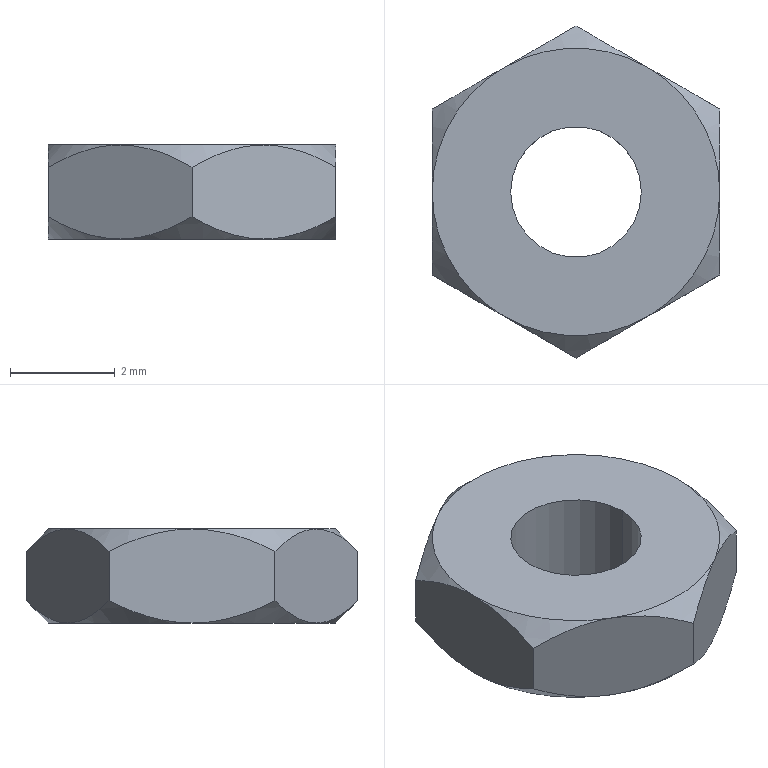Part | NX | 1 solid | 22 faces | box 5.5 x 6.351 x 1.8 mm | volume 37.693 mm3 | cone 12 | plane 8 | cylinder 2 | commonest cylinder face diameters 2.5 x2
STEP:
#1=CARTESIAN_POINT('',(1.375,-2.382,-0.9));
#2=VERTEX_POINT('',#1);
#3=CARTESIAN_POINT('',(2.75,0.,-0.9));
#4=VERTEX_POINT('',#3);
#5=CARTESIAN_POINT('',(0.,0.,-0.9));
#6=DIRECTION('',(0.,0.,1.));
#7=DIRECTION('',(0.5,-0.866,0.));
#8=AXIS2_PLACEMENT_3D('',#5,#6,#7);
#9=CIRCLE('',#8,2.75);
#10=EDGE_CURVE('',#2,#4,#9,.T.);
#11=ORIENTED_EDGE('',*,*,#10,.F.);
#12=CARTESIAN_POINT('',(-1.375,-2.382,-0.9));
#13=VERTEX_POINT('',#12);
#14=CARTESIAN_POINT('',(0.,0.,-0.9));
#15=DIRECTION('',(0.,0.,1.));
#16=DIRECTION('',(-0.5,-0.866,0.));
#17=AXIS2_PLACEMENT_3D('',#14,#15,#16);
#18=CIRCLE('',#17,2.75);
#19=EDGE_CURVE('',#13,#2,#18,.T.);
#20=ORIENTED_EDGE('',*,*,#19,.F.);
#21=CARTESIAN_POINT('',(-2.75,0.,-0.9));
#22=VERTEX_POINT('',#21);
#23=CARTESIAN_POINT('',(0.,0.,-0.9));
#24=DIRECTION('',(0.,0.,1.));
#25=DIRECTION('',(-1.,0.,0.));
#26=AXIS2_PLACEMENT_3D('',#23,#24,#25);
#27=CIRCLE('',#26,2.75);
#28=EDGE_CURVE('',#22,#13,#27,.T.);
#29=ORIENTED_EDGE('',*,*,#28,.F.);
#30=CARTESIAN_POINT('',(-1.375,2.382,-0.9));
#31=VERTEX_POINT('',#30);
#32=CARTESIAN_POINT('',(0.,0.,-0.9));
#33=DIRECTION('',(0.,0.,1.));
#34=DIRECTION('',(-0.5,0.866,0.));
#35=AXIS2_PLACEMENT_3D('',#32,#33,#34);
#36=CIRCLE('',#35,2.75);
#37=EDGE_CURVE('',#31,#22,#36,.T.);
#38=ORIENTED_EDGE('',*,*,#37,.F.);
#39=CARTESIAN_POINT('',(1.375,2.382,-0.9));
#40=VERTEX_POINT('',#39);
#41=CARTESIAN_POINT('',(0.,0.,-0.9));
#42=DIRECTION('',(0.,0.,1.));
#43=DIRECTION('',(0.5,0.866,0.));
#44=AXIS2_PLACEMENT_3D('',#41,#42,#43);
#45=CIRCLE('',#44,2.75);
#46=EDGE_CURVE('',#40,#31,#45,.T.);
#47=ORIENTED_EDGE('',*,*,#46,.F.);
#48=CARTESIAN_POINT('',(0.,0.,-0.9));
#49=DIRECTION('',(0.,0.,1.));
#50=DIRECTION('',(1.,0.,0.));
#51=AXIS2_PLACEMENT_3D('',#48,#49,#50);
#52=CIRCLE('',#51,2.75);
#53=EDGE_CURVE('',#4,#40,#52,.T.);
#54=ORIENTED_EDGE('',*,*,#53,.F.);
#55=EDGE_LOOP('',(#11,#20,#29,#38,#47,#54));
#56=FACE_BOUND('',#55,.T.);
#57=CARTESIAN_POINT('',(-1.25,0.,-0.9));
#58=VERTEX_POINT('',#57);
#59=CARTESIAN_POINT('',(1.25,0.,-0.9));
#60=VERTEX_POINT('',#59);
#61=CARTESIAN_POINT('',(0.,0.,-0.9));
#62=DIRECTION('',(0.,0.,-1.));
#63=DIRECTION('',(1.,0.,0.));
#64=AXIS2_PLACEMENT_3D('',#61,#62,#63);
#65=CIRCLE('',#64,1.25);
#66=EDGE_CURVE('',#58,#60,#65,.T.);
#67=ORIENTED_EDGE('',*,*,#66,.F.);
#68=CARTESIAN_POINT('',(0.,0.,-0.9));
#69=DIRECTION('',(0.,0.,-1.));
#70=DIRECTION('',(1.,0.,0.));
#71=AXIS2_PLACEMENT_3D('',#68,#69,#70);
#72=CIRCLE('',#71,1.25);
#73=EDGE_CURVE('',#60,#58,#72,.T.);
#74=ORIENTED_EDGE('',*,*,#73,.F.);
#75=EDGE_LOOP('',(#67,#74));
#76=FACE_BOUND('',#75,.T.);
#77=CARTESIAN_POINT('',(0.,0.,-0.9));
#78=DIRECTION('',(0.,0.,1.));
#79=DIRECTION('',(1.,0.,0.));
#80=AXIS2_PLACEMENT_3D('',#77,#78,#79);
#81=PLANE('',#80);
#82=ADVANCED_FACE('',(#56,#76),#81,.F.);
#83=CARTESIAN_POINT('',(2.75,-1.588,-0.4746));
#84=VERTEX_POINT('',#83);
#85=CARTESIAN_POINT('',(1.375,-2.382,-0.9));
#86=CARTESIAN_POINT('',(1.81,-2.131,-0.9));
#87=CARTESIAN_POINT('',(2.253,-1.875,-0.7618));
#88=CARTESIAN_POINT('',(2.75,-1.588,-0.4746));
#89=B_SPLINE_CURVE_WITH_KNOTS('',3,(#85,#86,#87,#88),.UNSPECIFIED.,.F.,.F.,(4,4),(0.,1.),.UNSPECIFIED.);
#90=EDGE_CURVE('',#2,#84,#89,.T.);
#91=ORIENTED_EDGE('',*,*,#90,.F.);
#92=ORIENTED_EDGE('',*,*,#10,.T.);
#93=CARTESIAN_POINT('',(2.75,-1.588,-0.4746));
#94=CARTESIAN_POINT('',(2.75,-1.016,-0.7606));
#95=CARTESIAN_POINT('',(2.75,-0.5054,-0.9));
#96=CARTESIAN_POINT('',(2.75,0.,-0.9));
#97=B_SPLINE_CURVE_WITH_KNOTS('',3,(#93,#94,#95,#96),.UNSPECIFIED.,.F.,.F.,(4,4),(0.,1.),.UNSPECIFIED.);
#98=EDGE_CURVE('',#84,#4,#97,.T.);
#99=ORIENTED_EDGE('',*,*,#98,.F.);
#100=EDGE_LOOP('',(#91,#92,#99));
#101=FACE_BOUND('',#100,.T.);
#102=CARTESIAN_POINT('',(0.,0.,-0.6873));
#103=DIRECTION('',(0.,0.,1.));
#104=DIRECTION('',(1.,0.,0.));
#105=AXIS2_PLACEMENT_3D('',#102,#103,#104);
#106=CONICAL_SURFACE('',#105,2.963,0.7854);
#107=ADVANCED_FACE('',(#101),#106,.T.);
#108=ORIENTED_EDGE('',*,*,#90,.T.);
#109=CARTESIAN_POINT('',(2.75,-1.588,0.4746));
#110=VERTEX_POINT('',#109);
#111=CARTESIAN_POINT('',(2.75,-1.588,0.4746));
#112=DIRECTION('',(0.,0.,-1.));
#113=VECTOR('',#112,1000.);
#114=LINE('',#111,#113);
#115=EDGE_CURVE('',#110,#84,#114,.T.);
#116=ORIENTED_EDGE('',*,*,#115,.F.);
#117=CARTESIAN_POINT('',(1.375,-2.382,0.9));
#118=VERTEX_POINT('',#117);
#119=CARTESIAN_POINT('',(2.75,-1.588,0.4746));
#120=CARTESIAN_POINT('',(2.529,-1.715,0.6022));
#121=CARTESIAN_POINT('',(2.163,-1.927,0.7878));
#122=CARTESIAN_POINT('',(1.617,-2.242,0.9));
#123=CARTESIAN_POINT('',(1.375,-2.382,0.9));
#124=B_SPLINE_CURVE_WITH_KNOTS('',3,(#119,#120,#121,#122,#123),.UNSPECIFIED.,.F.,.F.,(4,1,4),(0.,0.5,1.),.UNSPECIFIED.);
#125=EDGE_CURVE('',#118,#110,#124,.F.);
#126=ORIENTED_EDGE('',*,*,#125,.F.);
#127=CARTESIAN_POINT('',(0.,-3.175,0.4746));
#128=VERTEX_POINT('',#127);
#129=CARTESIAN_POINT('',(1.375,-2.382,0.9));
#130=CARTESIAN_POINT('',(0.9401,-2.633,0.9));
#131=CARTESIAN_POINT('',(0.4973,-2.888,0.7617));
#132=CARTESIAN_POINT('',(0.,-3.175,0.4746));
#133=B_SPLINE_CURVE_WITH_KNOTS('',3,(#129,#130,#131,#132),.UNSPECIFIED.,.F.,.F.,(4,4),(0.,1.),.UNSPECIFIED.);
#134=EDGE_CURVE('',#118,#128,#133,.T.);
#135=ORIENTED_EDGE('',*,*,#134,.T.);
#136=CARTESIAN_POINT('',(0.,-3.175,-0.4746));
#137=VERTEX_POINT('',#136);
#138=CARTESIAN_POINT('',(0.,-3.175,0.4746));
#139=DIRECTION('',(0.,0.,-1.));
#140=VECTOR('',#139,1000.);
#141=LINE('',#138,#140);
#142=EDGE_CURVE('',#128,#137,#141,.T.);
#143=ORIENTED_EDGE('',*,*,#142,.T.);
#144=CARTESIAN_POINT('',(0.,-3.175,-0.4746));
#145=CARTESIAN_POINT('',(0.05181,-3.146,-0.5045));
#146=CARTESIAN_POINT('',(0.1536,-3.087,-0.5607));
#147=CARTESIAN_POINT('',(0.3001,-3.002,-0.6342));
#148=CARTESIAN_POINT('',(0.4421,-2.92,-0.6978));
#149=CARTESIAN_POINT('',(0.5802,-2.84,-0.7522));
#150=CARTESIAN_POINT('',(0.7159,-2.762,-0.798));
#151=CARTESIAN_POINT('',(0.8496,-2.685,-0.8352));
#152=CARTESIAN_POINT('',(0.982,-2.608,-0.8642));
#153=CARTESIAN_POINT('',(1.113,-2.533,-0.8848));
#154=CARTESIAN_POINT('',(1.244,-2.457,-0.8972));
#155=CARTESIAN_POINT('',(1.331,-2.407,-0.9));
#156=CARTESIAN_POINT('',(1.375,-2.382,-0.9));
#157=B_SPLINE_CURVE_WITH_KNOTS('',3,(#144,#145,#146,#147,#148,#149,#150,#151,#152,#153,#154,#155,#156),.UNSPECIFIED.,.F.,.F.,(4,1,1,1,1,1,1,1,1,1,4),(0.,0.1,0.2,0.3,0.4,0.5,0.6,0.7,0.8,0.9,1.),.UNSPECIFIED.);
#158=EDGE_CURVE('',#137,#2,#157,.T.);
#159=ORIENTED_EDGE('',*,*,#158,.T.);
#160=EDGE_LOOP('',(#108,#116,#126,#135,#143,#159));
#161=FACE_BOUND('',#160,.T.);
#162=CARTESIAN_POINT('',(0.,-3.175,-0.9));
#163=DIRECTION('',(0.5,-0.866,0.));
#164=DIRECTION('',(0.,0.,-1.));
#165=AXIS2_PLACEMENT_3D('',#162,#163,#164);
#166=PLANE('',#165);
#167=ADVANCED_FACE('',(#161),#166,.T.);
#168=CARTESIAN_POINT('',(-1.375,-2.382,-0.9));
#169=CARTESIAN_POINT('',(-0.9404,-2.632,-0.9));
#170=CARTESIAN_POINT('',(-0.4974,-2.888,-0.7618));
#171=CARTESIAN_POINT('',(0.,-3.175,-0.4746));
#172=B_SPLINE_CURVE_WITH_KNOTS('',3,(#168,#169,#170,#171),.UNSPECIFIED.,.F.,.F.,(4,4),(0.,1.),.UNSPECIFIED.);
#173=EDGE_CURVE('',#13,#137,#172,.T.);
#174=ORIENTED_EDGE('',*,*,#173,.F.);
#175=ORIENTED_EDGE('',*,*,#19,.T.);
#176=ORIENTED_EDGE('',*,*,#158,.F.);
#177=EDGE_LOOP('',(#174,#175,#176));
#178=FACE_BOUND('',#177,.T.);
#179=CARTESIAN_POINT('',(0.,0.,-0.6873));
#180=DIRECTION('',(0.,0.,1.));
#181=DIRECTION('',(1.,0.,0.));
#182=AXIS2_PLACEMENT_3D('',#179,#180,#181);
#183=CONICAL_SURFACE('',#182,2.963,0.7854);
#184=ADVANCED_FACE('',(#178),#183,.T.);
#185=ORIENTED_EDGE('',*,*,#173,.T.);
#186=ORIENTED_EDGE('',*,*,#142,.F.);
#187=CARTESIAN_POINT('',(-1.375,-2.382,0.9));
#188=VERTEX_POINT('',#187);
#189=CARTESIAN_POINT('',(0.,-3.175,0.4746));
#190=CARTESIAN_POINT('',(-0.221,-3.048,0.6022));
#191=CARTESIAN_POINT('',(-0.5875,-2.836,0.7878));
#192=CARTESIAN_POINT('',(-1.133,-2.522,0.9));
#193=CARTESIAN_POINT('',(-1.375,-2.382,0.9));
#194=B_SPLINE_CURVE_WITH_KNOTS('',3,(#189,#190,#191,#192,#193),.UNSPECIFIED.,.F.,.F.,(4,1,4),(0.,0.5,1.),.UNSPECIFIED.);
#195=EDGE_CURVE('',#188,#128,#194,.F.);
#196=ORIENTED_EDGE('',*,*,#195,.F.);
#197=CARTESIAN_POINT('',(-2.75,-1.588,0.4746));
#198=VERTEX_POINT('',#197);
#199=CARTESIAN_POINT('',(-1.375,-2.382,0.9));
#200=CARTESIAN_POINT('',(-1.81,-2.131,0.9));
#201=CARTESIAN_POINT('',(-2.253,-1.875,0.7617));
#202=CARTESIAN_POINT('',(-2.75,-1.588,0.4746));
#203=B_SPLINE_CURVE_WITH_KNOTS('',3,(#199,#200,#201,#202),.UNSPECIFIED.,.F.,.F.,(4,4),(0.,1.),.UNSPECIFIED.);
#204=EDGE_CURVE('',#188,#198,#203,.T.);
#205=ORIENTED_EDGE('',*,*,#204,.T.);
#206=CARTESIAN_POINT('',(-2.75,-1.588,-0.4746));
#207=VERTEX_POINT('',#206);
#208=CARTESIAN_POINT('',(-2.75,-1.588,0.4746));
#209=DIRECTION('',(0.,0.,-1.));
#210=VECTOR('',#209,1000.);
#211=LINE('',#208,#210);
#212=EDGE_CURVE('',#198,#207,#211,.T.);
#213=ORIENTED_EDGE('',*,*,#212,.T.);
#214=CARTESIAN_POINT('',(-2.75,-1.588,-0.4746));
#215=CARTESIAN_POINT('',(-2.698,-1.618,-0.5045));
#216=CARTESIAN_POINT('',(-2.596,-1.676,-0.5607));
#217=CARTESIAN_POINT('',(-2.45,-1.761,-0.6342));
#218=CARTESIAN_POINT('',(-2.308,-1.843,-0.6978));
#219=CARTESIAN_POINT('',(-2.17,-1.923,-0.7522));
#220=CARTESIAN_POINT('',(-2.034,-2.001,-0.798));
#221=CARTESIAN_POINT('',(-1.9,-2.078,-0.8352));
#222=CARTESIAN_POINT('',(-1.768,-2.155,-0.8642));
#223=CARTESIAN_POINT('',(-1.637,-2.231,-0.8848));
#224=CARTESIAN_POINT('',(-1.506,-2.306,-0.8972));
#225=CARTESIAN_POINT('',(-1.419,-2.356,-0.9));
#226=CARTESIAN_POINT('',(-1.375,-2.382,-0.9));
#227=B_SPLINE_CURVE_WITH_KNOTS('',3,(#214,#215,#216,#217,#218,#219,#220,#221,#222,#223,#224,#225,#226),.UNSPECIFIED.,.F.,.F.,(4,1,1,1,1,1,1,1,1,1,4),(0.,0.1,0.2,0.3,0.4,0.5,0.6,0.7,0.8,0.9,1.),.UNSPECIFIED.);
#228=EDGE_CURVE('',#207,#13,#227,.T.);
#229=ORIENTED_EDGE('',*,*,#228,.T.);
#230=EDGE_LOOP('',(#185,#186,#196,#205,#213,#229));
#231=FACE_BOUND('',#230,.T.);
#232=CARTESIAN_POINT('',(-2.75,-1.588,-0.9));
#233=DIRECTION('',(-0.5,-0.866,0.));
#234=DIRECTION('',(-0.866,0.5,0.));
#235=AXIS2_PLACEMENT_3D('',#232,#233,#234);
#236=PLANE('',#235);
#237=ADVANCED_FACE('',(#231),#236,.T.);
#238=CARTESIAN_POINT('',(-2.75,0.,-0.9));
#239=CARTESIAN_POINT('',(-2.75,-0.5015,-0.9));
#240=CARTESIAN_POINT('',(-2.75,-1.013,-0.7618));
#241=CARTESIAN_POINT('',(-2.75,-1.588,-0.4746));
#242=B_SPLINE_CURVE_WITH_KNOTS('',3,(#238,#239,#240,#241),.UNSPECIFIED.,.F.,.F.,(4,4),(0.,1.),.UNSPECIFIED.);
#243=EDGE_CURVE('',#22,#207,#242,.T.);
#244=ORIENTED_EDGE('',*,*,#243,.F.);
#245=ORIENTED_EDGE('',*,*,#28,.T.);
#246=ORIENTED_EDGE('',*,*,#228,.F.);
#247=EDGE_LOOP('',(#244,#245,#246));
#248=FACE_BOUND('',#247,.T.);
#249=CARTESIAN_POINT('',(0.,0.,-0.6873));
#250=DIRECTION('',(0.,0.,1.));
#251=DIRECTION('',(1.,0.,0.));
#252=AXIS2_PLACEMENT_3D('',#249,#250,#251);
#253=CONICAL_SURFACE('',#252,2.963,0.7854);
#254=ADVANCED_FACE('',(#248),#253,.T.);
#255=ORIENTED_EDGE('',*,*,#243,.T.);
#256=ORIENTED_EDGE('',*,*,#212,.F.);
#257=CARTESIAN_POINT('',(-2.75,0.,0.9));
#258=VERTEX_POINT('',#257);
#259=CARTESIAN_POINT('',(-2.75,-1.588,0.4746));
#260=CARTESIAN_POINT('',(-2.75,-1.33,0.6035));
#261=CARTESIAN_POINT('',(-2.75,-0.8968,0.7916));
#262=CARTESIAN_POINT('',(-2.75,-0.2775,0.9));
#263=CARTESIAN_POINT('',(-2.75,0.,0.9));
#264=B_SPLINE_CURVE_WITH_KNOTS('',3,(#259,#260,#261,#262,#263),.UNSPECIFIED.,.F.,.F.,(4,1,4),(0.,0.5,1.),.UNSPECIFIED.);
#265=EDGE_CURVE('',#258,#198,#264,.F.);
#266=ORIENTED_EDGE('',*,*,#265,.F.);
#267=CARTESIAN_POINT('',(-2.75,1.588,0.4746));
#268=VERTEX_POINT('',#267);
#269=CARTESIAN_POINT('',(-2.75,0.,0.9));
#270=CARTESIAN_POINT('',(-2.75,0.5015,0.9));
#271=CARTESIAN_POINT('',(-2.75,1.013,0.7618));
#272=CARTESIAN_POINT('',(-2.75,1.588,0.4746));
#273=B_SPLINE_CURVE_WITH_KNOTS('',3,(#269,#270,#271,#272),.UNSPECIFIED.,.F.,.F.,(4,4),(0.,1.),.UNSPECIFIED.);
#274=EDGE_CURVE('',#258,#268,#273,.T.);
#275=ORIENTED_EDGE('',*,*,#274,.T.);
#276=CARTESIAN_POINT('',(-2.75,1.588,-0.4746));
#277=VERTEX_POINT('',#276);
#278=CARTESIAN_POINT('',(-2.75,1.588,0.4746));
#279=DIRECTION('',(0.,0.,-1.));
#280=VECTOR('',#279,1000.);
#281=LINE('',#278,#280);
#282=EDGE_CURVE('',#268,#277,#281,.T.);
#283=ORIENTED_EDGE('',*,*,#282,.T.);
#284=CARTESIAN_POINT('',(-2.75,1.588,-0.4746));
#285=CARTESIAN_POINT('',(-2.75,1.016,-0.7606));
#286=CARTESIAN_POINT('',(-2.75,0.5054,-0.9));
#287=CARTESIAN_POINT('',(-2.75,0.,-0.9));
#288=B_SPLINE_CURVE_WITH_KNOTS('',3,(#284,#285,#286,#287),.UNSPECIFIED.,.F.,.F.,(4,4),(0.,1.),.UNSPECIFIED.);
#289=EDGE_CURVE('',#277,#22,#288,.T.);
#290=ORIENTED_EDGE('',*,*,#289,.T.);
#291=EDGE_LOOP('',(#255,#256,#266,#275,#283,#290));
#292=FACE_BOUND('',#291,.T.);
#293=CARTESIAN_POINT('',(-2.75,1.588,-0.9));
#294=DIRECTION('',(-1.,0.,0.));
#295=DIRECTION('',(0.,0.,1.));
#296=AXIS2_PLACEMENT_3D('',#293,#294,#295);
#297=PLANE('',#296);
#298=ADVANCED_FACE('',(#292),#297,.T.);
#299=CARTESIAN_POINT('',(-1.375,2.382,-0.9));
#300=CARTESIAN_POINT('',(-1.81,2.131,-0.9));
#301=CARTESIAN_POINT('',(-2.253,1.875,-0.7618));
#302=CARTESIAN_POINT('',(-2.75,1.588,-0.4746));
#303=B_SPLINE_CURVE_WITH_KNOTS('',3,(#299,#300,#301,#302),.UNSPECIFIED.,.F.,.F.,(4,4),(0.,1.),.UNSPECIFIED.);
#304=EDGE_CURVE('',#31,#277,#303,.T.);
#305=ORIENTED_EDGE('',*,*,#304,.F.);
#306=ORIENTED_EDGE('',*,*,#37,.T.);
#307=ORIENTED_EDGE('',*,*,#289,.F.);
#308=EDGE_LOOP('',(#305,#306,#307));
#309=FACE_BOUND('',#308,.T.);
#310=CARTESIAN_POINT('',(0.,0.,-0.6873));
#311=DIRECTION('',(0.,0.,1.));
#312=DIRECTION('',(1.,0.,0.));
#313=AXIS2_PLACEMENT_3D('',#310,#311,#312);
#314=CONICAL_SURFACE('',#313,2.963,0.7854);
#315=ADVANCED_FACE('',(#309),#314,.T.);
#316=ORIENTED_EDGE('',*,*,#304,.T.);
#317=ORIENTED_EDGE('',*,*,#282,.F.);
#318=CARTESIAN_POINT('',(-1.375,2.382,0.9));
#319=VERTEX_POINT('',#318);
#320=CARTESIAN_POINT('',(-2.75,1.588,0.4746));
#321=CARTESIAN_POINT('',(-2.529,1.715,0.6022));
#322=CARTESIAN_POINT('',(-2.163,1.927,0.7878));
#323=CARTESIAN_POINT('',(-1.617,2.242,0.9));
#324=CARTESIAN_POINT('',(-1.375,2.382,0.9));
#325=B_SPLINE_CURVE_WITH_KNOTS('',3,(#320,#321,#322,#323,#324),.UNSPECIFIED.,.F.,.F.,(4,1,4),(0.,0.5,1.),.UNSPECIFIED.);
#326=EDGE_CURVE('',#319,#268,#325,.F.);
#327=ORIENTED_EDGE('',*,*,#326,.F.);
#328=CARTESIAN_POINT('',(0.,3.175,0.4746));
#329=VERTEX_POINT('',#328);
#330=CARTESIAN_POINT('',(-1.375,2.382,0.9));
#331=CARTESIAN_POINT('',(-0.9401,2.633,0.9));
#332=CARTESIAN_POINT('',(-0.4973,2.888,0.7617));
#333=CARTESIAN_POINT('',(0.,3.175,0.4746));
#334=B_SPLINE_CURVE_WITH_KNOTS('',3,(#330,#331,#332,#333),.UNSPECIFIED.,.F.,.F.,(4,4),(0.,1.),.UNSPECIFIED.);
#335=EDGE_CURVE('',#319,#329,#334,.T.);
#336=ORIENTED_EDGE('',*,*,#335,.T.);
#337=CARTESIAN_POINT('',(0.,3.175,-0.4746));
#338=VERTEX_POINT('',#337);
#339=CARTESIAN_POINT('',(0.,3.175,0.4746));
#340=DIRECTION('',(0.,0.,-1.));
#341=VECTOR('',#340,1000.);
#342=LINE('',#339,#341);
#343=EDGE_CURVE('',#329,#338,#342,.T.);
#344=ORIENTED_EDGE('',*,*,#343,.T.);
#345=CARTESIAN_POINT('',(0.,3.175,-0.4746));
#346=CARTESIAN_POINT('',(-0.05181,3.146,-0.5045));
#347=CARTESIAN_POINT('',(-0.1536,3.087,-0.5607));
#348=CARTESIAN_POINT('',(-0.3001,3.002,-0.6342));
#349=CARTESIAN_POINT('',(-0.4421,2.92,-0.6978));
#350=CARTESIAN_POINT('',(-0.5802,2.84,-0.7522));
#351=CARTESIAN_POINT('',(-0.7159,2.762,-0.798));
#352=CARTESIAN_POINT('',(-0.8496,2.685,-0.8352));
#353=CARTESIAN_POINT('',(-0.982,2.608,-0.8642));
#354=CARTESIAN_POINT('',(-1.113,2.533,-0.8848));
#355=CARTESIAN_POINT('',(-1.244,2.457,-0.8972));
#356=CARTESIAN_POINT('',(-1.331,2.407,-0.9));
#357=CARTESIAN_POINT('',(-1.375,2.382,-0.9));
#358=B_SPLINE_CURVE_WITH_KNOTS('',3,(#345,#346,#347,#348,#349,#350,#351,#352,#353,#354,#355,#356,#357),.UNSPECIFIED.,.F.,.F.,(4,1,1,1,1,1,1,1,1,1,4),(0.,0.1,0.2,0.3,0.4,0.5,0.6,0.7,0.8,0.9,1.),.UNSPECIFIED.);
#359=EDGE_CURVE('',#338,#31,#358,.T.);
#360=ORIENTED_EDGE('',*,*,#359,.T.);
#361=EDGE_LOOP('',(#316,#317,#327,#336,#344,#360));
#362=FACE_BOUND('',#361,.T.);
#363=CARTESIAN_POINT('',(0.,3.175,-0.9));
#364=DIRECTION('',(-0.5,0.866,0.));
#365=DIRECTION('',(0.,0.,1.));
#366=AXIS2_PLACEMENT_3D('',#363,#364,#365);
#367=PLANE('',#366);
#368=ADVANCED_FACE('',(#362),#367,.T.);
#369=CARTESIAN_POINT('',(1.375,2.382,-0.9));
#370=CARTESIAN_POINT('',(0.9404,2.632,-0.9));
#371=CARTESIAN_POINT('',(0.4974,2.888,-0.7618));
#372=CARTESIAN_POINT('',(0.,3.175,-0.4746));
#373=B_SPLINE_CURVE_WITH_KNOTS('',3,(#369,#370,#371,#372),.UNSPECIFIED.,.F.,.F.,(4,4),(0.,1.),.UNSPECIFIED.);
#374=EDGE_CURVE('',#40,#338,#373,.T.);
#375=ORIENTED_EDGE('',*,*,#374,.F.);
#376=ORIENTED_EDGE('',*,*,#46,.T.);
#377=ORIENTED_EDGE('',*,*,#359,.F.);
#378=EDGE_LOOP('',(#375,#376,#377));
#379=FACE_BOUND('',#378,.T.);
#380=CARTESIAN_POINT('',(0.,0.,-0.6873));
#381=DIRECTION('',(0.,0.,1.));
#382=DIRECTION('',(1.,0.,0.));
#383=AXIS2_PLACEMENT_3D('',#380,#381,#382);
#384=CONICAL_SURFACE('',#383,2.963,0.7854);
#385=ADVANCED_FACE('',(#379),#384,.T.);
#386=ORIENTED_EDGE('',*,*,#374,.T.);
#387=ORIENTED_EDGE('',*,*,#343,.F.);
#388=CARTESIAN_POINT('',(1.375,2.382,0.9));
#389=VERTEX_POINT('',#388);
#390=CARTESIAN_POINT('',(0.,3.175,0.4746));
#391=CARTESIAN_POINT('',(0.221,3.048,0.6022));
#392=CARTESIAN_POINT('',(0.5875,2.836,0.7878));
#393=CARTESIAN_POINT('',(1.133,2.522,0.9));
#394=CARTESIAN_POINT('',(1.375,2.382,0.9));
#395=B_SPLINE_CURVE_WITH_KNOTS('',3,(#390,#391,#392,#393,#394),.UNSPECIFIED.,.F.,.F.,(4,1,4),(0.,0.5,1.),.UNSPECIFIED.);
#396=EDGE_CURVE('',#389,#329,#395,.F.);
#397=ORIENTED_EDGE('',*,*,#396,.F.);
#398=CARTESIAN_POINT('',(2.75,1.588,0.4746));
#399=VERTEX_POINT('',#398);
#400=CARTESIAN_POINT('',(1.375,2.382,0.9));
#401=CARTESIAN_POINT('',(1.81,2.131,0.9));
#402=CARTESIAN_POINT('',(2.253,1.875,0.7617));
#403=CARTESIAN_POINT('',(2.75,1.588,0.4746));
#404=B_SPLINE_CURVE_WITH_KNOTS('',3,(#400,#401,#402,#403),.UNSPECIFIED.,.F.,.F.,(4,4),(0.,1.),.UNSPECIFIED.);
#405=EDGE_CURVE('',#389,#399,#404,.T.);
#406=ORIENTED_EDGE('',*,*,#405,.T.);
#407=CARTESIAN_POINT('',(2.75,1.588,-0.4746));
#408=VERTEX_POINT('',#407);
#409=CARTESIAN_POINT('',(2.75,1.588,0.4746));
#410=DIRECTION('',(0.,0.,-1.));
#411=VECTOR('',#410,1000.);
#412=LINE('',#409,#411);
#413=EDGE_CURVE('',#399,#408,#412,.T.);
#414=ORIENTED_EDGE('',*,*,#413,.T.);
#415=CARTESIAN_POINT('',(2.75,1.588,-0.4746));
#416=CARTESIAN_POINT('',(2.698,1.618,-0.5045));
#417=CARTESIAN_POINT('',(2.596,1.676,-0.5607));
#418=CARTESIAN_POINT('',(2.45,1.761,-0.6342));
#419=CARTESIAN_POINT('',(2.308,1.843,-0.6978));
#420=CARTESIAN_POINT('',(2.17,1.923,-0.7522));
#421=CARTESIAN_POINT('',(2.034,2.001,-0.798));
#422=CARTESIAN_POINT('',(1.9,2.078,-0.8352));
#423=CARTESIAN_POINT('',(1.768,2.155,-0.8642));
#424=CARTESIAN_POINT('',(1.637,2.231,-0.8848));
#425=CARTESIAN_POINT('',(1.506,2.306,-0.8972));
#426=CARTESIAN_POINT('',(1.419,2.356,-0.9));
#427=CARTESIAN_POINT('',(1.375,2.382,-0.9));
#428=B_SPLINE_CURVE_WITH_KNOTS('',3,(#415,#416,#417,#418,#419,#420,#421,#422,#423,#424,#425,#426,#427),.UNSPECIFIED.,.F.,.F.,(4,1,1,1,1,1,1,1,1,1,4),(0.,0.1,0.2,0.3,0.4,0.5,0.6,0.7,0.8,0.9,1.),.UNSPECIFIED.);
#429=EDGE_CURVE('',#408,#40,#428,.T.);
#430=ORIENTED_EDGE('',*,*,#429,.T.);
#431=EDGE_LOOP('',(#386,#387,#397,#406,#414,#430));
#432=FACE_BOUND('',#431,.T.);
#433=CARTESIAN_POINT('',(2.75,1.588,-0.9));
#434=DIRECTION('',(0.5,0.866,0.));
#435=DIRECTION('',(0.,0.,-1.));
#436=AXIS2_PLACEMENT_3D('',#433,#434,#435);
#437=PLANE('',#436);
#438=ADVANCED_FACE('',(#432),#437,.T.);
#439=CARTESIAN_POINT('',(2.75,0.,-0.9));
#440=CARTESIAN_POINT('',(2.75,0.5015,-0.9));
#441=CARTESIAN_POINT('',(2.75,1.013,-0.7618));
#442=CARTESIAN_POINT('',(2.75,1.588,-0.4746));
#443=B_SPLINE_CURVE_WITH_KNOTS('',3,(#439,#440,#441,#442),.UNSPECIFIED.,.F.,.F.,(4,4),(0.,1.),.UNSPECIFIED.);
#444=EDGE_CURVE('',#4,#408,#443,.T.);
#445=ORIENTED_EDGE('',*,*,#444,.F.);
#446=ORIENTED_EDGE('',*,*,#53,.T.);
#447=ORIENTED_EDGE('',*,*,#429,.F.);
#448=EDGE_LOOP('',(#445,#446,#447));
#449=FACE_BOUND('',#448,.T.);
#450=CARTESIAN_POINT('',(0.,0.,-0.6873));
#451=DIRECTION('',(0.,0.,1.));
#452=DIRECTION('',(1.,0.,0.));
#453=AXIS2_PLACEMENT_3D('',#450,#451,#452);
#454=CONICAL_SURFACE('',#453,2.963,0.7854);
#455=ADVANCED_FACE('',(#449),#454,.T.);
#456=ORIENTED_EDGE('',*,*,#98,.T.);
#457=ORIENTED_EDGE('',*,*,#444,.T.);
#458=ORIENTED_EDGE('',*,*,#413,.F.);
#459=CARTESIAN_POINT('',(2.75,0.,0.9));
#460=VERTEX_POINT('',#459);
#461=CARTESIAN_POINT('',(2.75,1.588,0.4746));
#462=CARTESIAN_POINT('',(2.75,1.33,0.6035));
#463=CARTESIAN_POINT('',(2.75,0.8968,0.7916));
#464=CARTESIAN_POINT('',(2.75,0.2775,0.9));
#465=CARTESIAN_POINT('',(2.75,0.,0.9));
#466=B_SPLINE_CURVE_WITH_KNOTS('',3,(#461,#462,#463,#464,#465),.UNSPECIFIED.,.F.,.F.,(4,1,4),(0.,0.5,1.),.UNSPECIFIED.);
#467=EDGE_CURVE('',#460,#399,#466,.F.);
#468=ORIENTED_EDGE('',*,*,#467,.F.);
#469=CARTESIAN_POINT('',(2.75,0.,0.9));
#470=CARTESIAN_POINT('',(2.75,-0.5015,0.9));
#471=CARTESIAN_POINT('',(2.75,-1.013,0.7618));
#472=CARTESIAN_POINT('',(2.75,-1.588,0.4746));
#473=B_SPLINE_CURVE_WITH_KNOTS('',3,(#469,#470,#471,#472),.UNSPECIFIED.,.F.,.F.,(4,4),(0.,1.),.UNSPECIFIED.);
#474=EDGE_CURVE('',#460,#110,#473,.T.);
#475=ORIENTED_EDGE('',*,*,#474,.T.);
#476=ORIENTED_EDGE('',*,*,#115,.T.);
#477=EDGE_LOOP('',(#456,#457,#458,#468,#475,#476));
#478=FACE_BOUND('',#477,.T.);
#479=CARTESIAN_POINT('',(2.75,-1.588,-0.9));
#480=DIRECTION('',(1.,0.,0.));
#481=DIRECTION('',(0.,1.,0.));
#482=AXIS2_PLACEMENT_3D('',#479,#480,#481);
#483=PLANE('',#482);
#484=ADVANCED_FACE('',(#478),#483,.T.);
#485=ORIENTED_EDGE('',*,*,#474,.F.);
#486=CARTESIAN_POINT('',(0.,0.,0.9));
#487=DIRECTION('',(0.,0.,-1.));
#488=DIRECTION('',(1.,0.,0.));
#489=AXIS2_PLACEMENT_3D('',#486,#487,#488);
#490=CIRCLE('',#489,2.75);
#491=EDGE_CURVE('',#460,#118,#490,.T.);
#492=ORIENTED_EDGE('',*,*,#491,.T.);
#493=ORIENTED_EDGE('',*,*,#125,.T.);
#494=EDGE_LOOP('',(#485,#492,#493));
#495=FACE_BOUND('',#494,.T.);
#496=CARTESIAN_POINT('',(0.,0.,0.6873));
#497=DIRECTION('',(0.,0.,-1.));
#498=DIRECTION('',(-1.,0.,0.));
#499=AXIS2_PLACEMENT_3D('',#496,#497,#498);
#500=CONICAL_SURFACE('',#499,2.963,0.7854);
#501=ADVANCED_FACE('',(#495),#500,.T.);
#502=ORIENTED_EDGE('',*,*,#491,.F.);
#503=CARTESIAN_POINT('',(0.,0.,0.9));
#504=DIRECTION('',(0.,0.,-1.));
#505=DIRECTION('',(0.5,0.866,0.));
#506=AXIS2_PLACEMENT_3D('',#503,#504,#505);
#507=CIRCLE('',#506,2.75);
#508=EDGE_CURVE('',#389,#460,#507,.T.);
#509=ORIENTED_EDGE('',*,*,#508,.F.);
#510=CARTESIAN_POINT('',(0.,0.,0.9));
#511=DIRECTION('',(0.,0.,-1.));
#512=DIRECTION('',(-0.5,0.866,0.));
#513=AXIS2_PLACEMENT_3D('',#510,#511,#512);
#514=CIRCLE('',#513,2.75);
#515=EDGE_CURVE('',#319,#389,#514,.T.);
#516=ORIENTED_EDGE('',*,*,#515,.F.);
#517=CARTESIAN_POINT('',(0.,0.,0.9));
#518=DIRECTION('',(0.,0.,-1.));
#519=DIRECTION('',(-1.,0.,0.));
#520=AXIS2_PLACEMENT_3D('',#517,#518,#519);
#521=CIRCLE('',#520,2.75);
#522=EDGE_CURVE('',#258,#319,#521,.T.);
#523=ORIENTED_EDGE('',*,*,#522,.F.);
#524=CARTESIAN_POINT('',(0.,0.,0.9));
#525=DIRECTION('',(0.,0.,-1.));
#526=DIRECTION('',(-0.5,-0.866,0.));
#527=AXIS2_PLACEMENT_3D('',#524,#525,#526);
#528=CIRCLE('',#527,2.75);
#529=EDGE_CURVE('',#188,#258,#528,.T.);
#530=ORIENTED_EDGE('',*,*,#529,.F.);
#531=CARTESIAN_POINT('',(0.,0.,0.9));
#532=DIRECTION('',(0.,0.,-1.));
#533=DIRECTION('',(0.5,-0.866,0.));
#534=AXIS2_PLACEMENT_3D('',#531,#532,#533);
#535=CIRCLE('',#534,2.75);
#536=EDGE_CURVE('',#118,#188,#535,.T.);
#537=ORIENTED_EDGE('',*,*,#536,.F.);
#538=EDGE_LOOP('',(#502,#509,#516,#523,#530,#537));
#539=FACE_BOUND('',#538,.T.);
#540=CARTESIAN_POINT('',(1.25,0.,0.9));
#541=VERTEX_POINT('',#540);
#542=CARTESIAN_POINT('',(-1.25,0.,0.9));
#543=VERTEX_POINT('',#542);
#544=CARTESIAN_POINT('',(0.,0.,0.9));
#545=DIRECTION('',(0.,0.,1.));
#546=DIRECTION('',(-1.,0.,0.));
#547=AXIS2_PLACEMENT_3D('',#544,#545,#546);
#548=CIRCLE('',#547,1.25);
#549=EDGE_CURVE('',#541,#543,#548,.T.);
#550=ORIENTED_EDGE('',*,*,#549,.F.);
#551=CARTESIAN_POINT('',(0.,0.,0.9));
#552=DIRECTION('',(0.,0.,1.));
#553=DIRECTION('',(-1.,0.,0.));
#554=AXIS2_PLACEMENT_3D('',#551,#552,#553);
#555=CIRCLE('',#554,1.25);
#556=EDGE_CURVE('',#543,#541,#555,.T.);
#557=ORIENTED_EDGE('',*,*,#556,.F.);
#558=EDGE_LOOP('',(#550,#557));
#559=FACE_BOUND('',#558,.T.);
#560=CARTESIAN_POINT('',(0.,0.,0.9));
#561=DIRECTION('',(0.,0.,1.));
#562=DIRECTION('',(1.,0.,0.));
#563=AXIS2_PLACEMENT_3D('',#560,#561,#562);
#564=PLANE('',#563);
#565=ADVANCED_FACE('',(#539,#559),#564,.T.);
#566=ORIENTED_EDGE('',*,*,#134,.F.);
#567=ORIENTED_EDGE('',*,*,#536,.T.);
#568=ORIENTED_EDGE('',*,*,#195,.T.);
#569=EDGE_LOOP('',(#566,#567,#568));
#570=FACE_BOUND('',#569,.T.);
#571=CARTESIAN_POINT('',(0.,0.,0.6873));
#572=DIRECTION('',(0.,0.,-1.));
#573=DIRECTION('',(-1.,0.,0.));
#574=AXIS2_PLACEMENT_3D('',#571,#572,#573);
#575=CONICAL_SURFACE('',#574,2.963,0.7854);
#576=ADVANCED_FACE('',(#570),#575,.T.);
#577=ORIENTED_EDGE('',*,*,#204,.F.);
#578=ORIENTED_EDGE('',*,*,#529,.T.);
#579=ORIENTED_EDGE('',*,*,#265,.T.);
#580=EDGE_LOOP('',(#577,#578,#579));
#581=FACE_BOUND('',#580,.T.);
#582=CARTESIAN_POINT('',(0.,0.,0.6873));
#583=DIRECTION('',(0.,0.,-1.));
#584=DIRECTION('',(-1.,0.,0.));
#585=AXIS2_PLACEMENT_3D('',#582,#583,#584);
#586=CONICAL_SURFACE('',#585,2.963,0.7854);
#587=ADVANCED_FACE('',(#581),#586,.T.);
#588=ORIENTED_EDGE('',*,*,#274,.F.);
#589=ORIENTED_EDGE('',*,*,#522,.T.);
#590=ORIENTED_EDGE('',*,*,#326,.T.);
#591=EDGE_LOOP('',(#588,#589,#590));
#592=FACE_BOUND('',#591,.T.);
#593=CARTESIAN_POINT('',(0.,0.,0.6873));
#594=DIRECTION('',(0.,0.,-1.));
#595=DIRECTION('',(-1.,0.,0.));
#596=AXIS2_PLACEMENT_3D('',#593,#594,#595);
#597=CONICAL_SURFACE('',#596,2.963,0.7854);
#598=ADVANCED_FACE('',(#592),#597,.T.);
#599=ORIENTED_EDGE('',*,*,#335,.F.);
#600=ORIENTED_EDGE('',*,*,#515,.T.);
#601=ORIENTED_EDGE('',*,*,#396,.T.);
#602=EDGE_LOOP('',(#599,#600,#601));
#603=FACE_BOUND('',#602,.T.);
#604=CARTESIAN_POINT('',(0.,0.,0.6873));
#605=DIRECTION('',(0.,0.,-1.));
#606=DIRECTION('',(-1.,0.,0.));
#607=AXIS2_PLACEMENT_3D('',#604,#605,#606);
#608=CONICAL_SURFACE('',#607,2.963,0.7854);
#609=ADVANCED_FACE('',(#603),#608,.T.);
#610=ORIENTED_EDGE('',*,*,#405,.F.);
#611=ORIENTED_EDGE('',*,*,#508,.T.);
#612=ORIENTED_EDGE('',*,*,#467,.T.);
#613=EDGE_LOOP('',(#610,#611,#612));
#614=FACE_BOUND('',#613,.T.);
#615=CARTESIAN_POINT('',(0.,0.,0.6873));
#616=DIRECTION('',(0.,0.,-1.));
#617=DIRECTION('',(-1.,0.,0.));
#618=AXIS2_PLACEMENT_3D('',#615,#616,#617);
#619=CONICAL_SURFACE('',#618,2.963,0.7854);
#620=ADVANCED_FACE('',(#614),#619,.T.);
#621=ORIENTED_EDGE('',*,*,#549,.T.);
#622=CARTESIAN_POINT('',(-1.25,0.,0.9));
#623=DIRECTION('',(0.,0.,-1.));
#624=VECTOR('',#623,1000.);
#625=LINE('',#622,#624);
#626=EDGE_CURVE('',#58,#543,#625,.F.);
#627=ORIENTED_EDGE('',*,*,#626,.F.);
#628=ORIENTED_EDGE('',*,*,#66,.T.);
#629=CARTESIAN_POINT('',(1.25,0.,0.9));
#630=DIRECTION('',(0.,0.,-1.));
#631=VECTOR('',#630,1000.);
#632=LINE('',#629,#631);
#633=EDGE_CURVE('',#60,#541,#632,.F.);
#634=ORIENTED_EDGE('',*,*,#633,.T.);
#635=EDGE_LOOP('',(#621,#627,#628,#634));
#636=FACE_BOUND('',#635,.T.);
#637=CARTESIAN_POINT('',(0.,0.,0.9));
#638=DIRECTION('',(0.,0.,-1.));
#639=DIRECTION('',(-1.,0.,0.));
#640=AXIS2_PLACEMENT_3D('',#637,#638,#639);
#641=CYLINDRICAL_SURFACE('',#640,1.25);
#642=ADVANCED_FACE('',(#636),#641,.F.);
#643=ORIENTED_EDGE('',*,*,#626,.T.);
#644=ORIENTED_EDGE('',*,*,#556,.T.);
#645=ORIENTED_EDGE('',*,*,#633,.F.);
#646=ORIENTED_EDGE('',*,*,#73,.T.);
#647=EDGE_LOOP('',(#643,#644,#645,#646));
#648=FACE_BOUND('',#647,.T.);
#649=CARTESIAN_POINT('',(0.,0.,0.9));
#650=DIRECTION('',(0.,0.,-1.));
#651=DIRECTION('',(-1.,0.,0.));
#652=AXIS2_PLACEMENT_3D('',#649,#650,#651);
#653=CYLINDRICAL_SURFACE('',#652,1.25);
#654=ADVANCED_FACE('',(#648),#653,.F.);
#655=CLOSED_SHELL('',(#82,#107,#167,#184,#237,#254,#298,#315,#368,#385,#438,#455,#484,#501,#565,#576,#587,#598,#609,#620,#642,#654));
#656=MANIFOLD_SOLID_BREP('',#655);
#657=(LENGTH_UNIT()NAMED_UNIT(*)SI_UNIT(.MILLI.,.METRE.));
#658=UNCERTAINTY_MEASURE_WITH_UNIT(LENGTH_MEASURE(0.0508),#657,'','');
#659=(NAMED_UNIT(*)PLANE_ANGLE_UNIT()SI_UNIT($,.RADIAN.));
#660=(NAMED_UNIT(*)SI_UNIT($,.STERADIAN.)SOLID_ANGLE_UNIT());
#661=(GEOMETRIC_REPRESENTATION_CONTEXT(3)GLOBAL_UNCERTAINTY_ASSIGNED_CONTEXT((#658))GLOBAL_UNIT_ASSIGNED_CONTEXT((#657,#659,#660))REPRESENTATION_CONTEXT('',''));
#662=ADVANCED_BREP_SHAPE_REPRESENTATION('',(#656),#661);